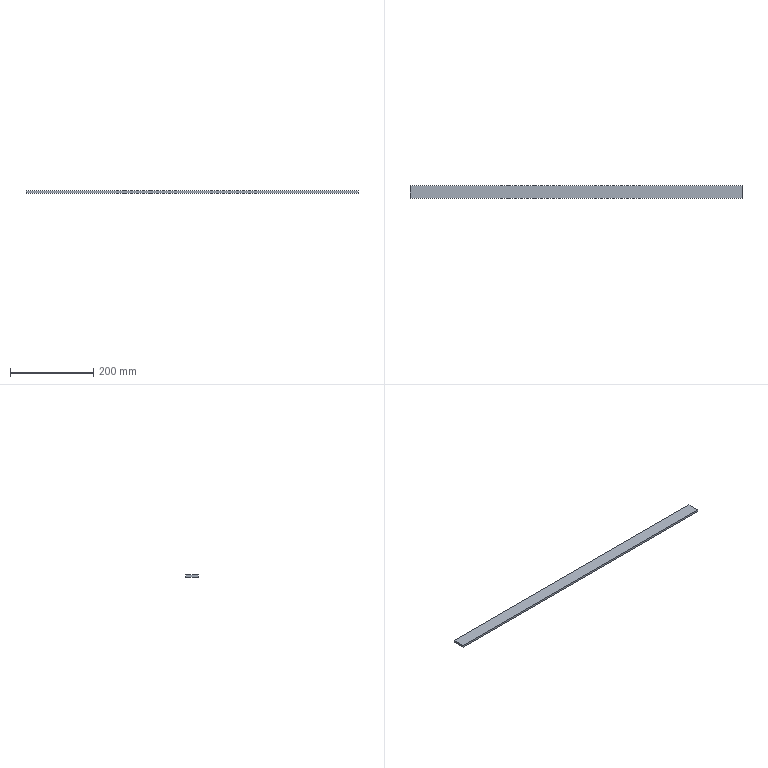Part | SolidWorks | features Extrusion 1 | 1 solid | 6 faces | box 800 x 30 x 5 mm | volume 120000 mm3 | plane 6
STEP:
#1=CARTESIAN_POINT('',(400.,-15.,0.));
#2=VERTEX_POINT('',#1);
#3=CARTESIAN_POINT('',(400.,15.,0.));
#4=VERTEX_POINT('',#3);
#5=CARTESIAN_POINT('',(400.,15.,0.));
#6=DIRECTION('',(0.,1.,0.));
#7=VECTOR('',#6,1000.);
#8=LINE('',#5,#7);
#9=EDGE_CURVE('',#2,#4,#8,.T.);
#10=ORIENTED_EDGE('',*,*,#9,.T.);
#11=CARTESIAN_POINT('',(400.,15.,5.));
#12=VERTEX_POINT('',#11);
#13=CARTESIAN_POINT('',(400.,15.,5.));
#14=DIRECTION('',(0.,0.,-1.));
#15=VECTOR('',#14,1000.);
#16=LINE('',#13,#15);
#17=EDGE_CURVE('',#12,#4,#16,.T.);
#18=ORIENTED_EDGE('',*,*,#17,.F.);
#19=CARTESIAN_POINT('',(400.,-15.,5.));
#20=VERTEX_POINT('',#19);
#21=CARTESIAN_POINT('',(400.,15.,5.));
#22=DIRECTION('',(0.,1.,0.));
#23=VECTOR('',#22,1000.);
#24=LINE('',#21,#23);
#25=EDGE_CURVE('',#20,#12,#24,.T.);
#26=ORIENTED_EDGE('',*,*,#25,.F.);
#27=CARTESIAN_POINT('',(400.,-15.,5.));
#28=DIRECTION('',(0.,0.,-1.));
#29=VECTOR('',#28,1000.);
#30=LINE('',#27,#29);
#31=EDGE_CURVE('',#20,#2,#30,.T.);
#32=ORIENTED_EDGE('',*,*,#31,.T.);
#33=EDGE_LOOP('',(#10,#18,#26,#32));
#34=FACE_OUTER_BOUND('',#33,.T.);
#35=CARTESIAN_POINT('',(400.,15.,5.));
#36=DIRECTION('',(-1.,0.,0.));
#37=DIRECTION('',(0.,0.,1.));
#38=AXIS2_PLACEMENT_3D('',#35,#36,#37);
#39=PLANE('',#38);
#40=ADVANCED_FACE('',(#34),#39,.F.);
#41=CARTESIAN_POINT('',(-400.,15.,0.));
#42=VERTEX_POINT('',#41);
#43=CARTESIAN_POINT('',(-400.,15.,0.));
#44=DIRECTION('',(-1.,0.,0.));
#45=VECTOR('',#44,1000.);
#46=LINE('',#43,#45);
#47=EDGE_CURVE('',#4,#42,#46,.T.);
#48=ORIENTED_EDGE('',*,*,#47,.T.);
#49=CARTESIAN_POINT('',(-400.,15.,5.));
#50=VERTEX_POINT('',#49);
#51=CARTESIAN_POINT('',(-400.,15.,5.));
#52=DIRECTION('',(0.,0.,-1.));
#53=VECTOR('',#52,1000.);
#54=LINE('',#51,#53);
#55=EDGE_CURVE('',#50,#42,#54,.T.);
#56=ORIENTED_EDGE('',*,*,#55,.F.);
#57=CARTESIAN_POINT('',(-400.,15.,5.));
#58=DIRECTION('',(-1.,0.,0.));
#59=VECTOR('',#58,1000.);
#60=LINE('',#57,#59);
#61=EDGE_CURVE('',#12,#50,#60,.T.);
#62=ORIENTED_EDGE('',*,*,#61,.F.);
#63=ORIENTED_EDGE('',*,*,#17,.T.);
#64=EDGE_LOOP('',(#48,#56,#62,#63));
#65=FACE_OUTER_BOUND('',#64,.T.);
#66=CARTESIAN_POINT('',(-400.,15.,5.));
#67=DIRECTION('',(0.,-1.,0.));
#68=DIRECTION('',(0.,0.,-1.));
#69=AXIS2_PLACEMENT_3D('',#66,#67,#68);
#70=PLANE('',#69);
#71=ADVANCED_FACE('',(#65),#70,.F.);
#72=CARTESIAN_POINT('',(-400.,-15.,0.));
#73=VERTEX_POINT('',#72);
#74=CARTESIAN_POINT('',(-400.,15.,0.));
#75=DIRECTION('',(0.,-1.,0.));
#76=VECTOR('',#75,1000.);
#77=LINE('',#74,#76);
#78=EDGE_CURVE('',#42,#73,#77,.T.);
#79=ORIENTED_EDGE('',*,*,#78,.T.);
#80=CARTESIAN_POINT('',(-400.,-15.,5.));
#81=VERTEX_POINT('',#80);
#82=CARTESIAN_POINT('',(-400.,-15.,5.));
#83=DIRECTION('',(0.,0.,-1.));
#84=VECTOR('',#83,1000.);
#85=LINE('',#82,#84);
#86=EDGE_CURVE('',#81,#73,#85,.T.);
#87=ORIENTED_EDGE('',*,*,#86,.F.);
#88=CARTESIAN_POINT('',(-400.,15.,5.));
#89=DIRECTION('',(0.,-1.,0.));
#90=VECTOR('',#89,1000.);
#91=LINE('',#88,#90);
#92=EDGE_CURVE('',#50,#81,#91,.T.);
#93=ORIENTED_EDGE('',*,*,#92,.F.);
#94=ORIENTED_EDGE('',*,*,#55,.T.);
#95=EDGE_LOOP('',(#79,#87,#93,#94));
#96=FACE_OUTER_BOUND('',#95,.T.);
#97=CARTESIAN_POINT('',(-400.,15.,5.));
#98=DIRECTION('',(1.,0.,0.));
#99=DIRECTION('',(0.,0.,-1.));
#100=AXIS2_PLACEMENT_3D('',#97,#98,#99);
#101=PLANE('',#100);
#102=ADVANCED_FACE('',(#96),#101,.F.);
#103=CARTESIAN_POINT('',(-400.,-15.,0.));
#104=DIRECTION('',(1.,0.,0.));
#105=VECTOR('',#104,1000.);
#106=LINE('',#103,#105);
#107=EDGE_CURVE('',#73,#2,#106,.T.);
#108=ORIENTED_EDGE('',*,*,#107,.T.);
#109=ORIENTED_EDGE('',*,*,#31,.F.);
#110=CARTESIAN_POINT('',(-400.,-15.,5.));
#111=DIRECTION('',(1.,0.,0.));
#112=VECTOR('',#111,1000.);
#113=LINE('',#110,#112);
#114=EDGE_CURVE('',#81,#20,#113,.T.);
#115=ORIENTED_EDGE('',*,*,#114,.F.);
#116=ORIENTED_EDGE('',*,*,#86,.T.);
#117=EDGE_LOOP('',(#108,#109,#115,#116));
#118=FACE_OUTER_BOUND('',#117,.T.);
#119=CARTESIAN_POINT('',(-400.,-15.,5.));
#120=DIRECTION('',(0.,1.,0.));
#121=DIRECTION('',(0.,0.,1.));
#122=AXIS2_PLACEMENT_3D('',#119,#120,#121);
#123=PLANE('',#122);
#124=ADVANCED_FACE('',(#118),#123,.F.);
#125=ORIENTED_EDGE('',*,*,#25,.T.);
#126=ORIENTED_EDGE('',*,*,#61,.T.);
#127=ORIENTED_EDGE('',*,*,#92,.T.);
#128=ORIENTED_EDGE('',*,*,#114,.T.);
#129=EDGE_LOOP('',(#125,#126,#127,#128));
#130=FACE_OUTER_BOUND('',#129,.T.);
#131=CARTESIAN_POINT('',(0.,0.,5.));
#132=DIRECTION('',(0.,0.,1.));
#133=DIRECTION('',(1.,0.,0.));
#134=AXIS2_PLACEMENT_3D('',#131,#132,#133);
#135=PLANE('',#134);
#136=ADVANCED_FACE('',(#130),#135,.T.);
#137=ORIENTED_EDGE('',*,*,#9,.F.);
#138=ORIENTED_EDGE('',*,*,#107,.F.);
#139=ORIENTED_EDGE('',*,*,#78,.F.);
#140=ORIENTED_EDGE('',*,*,#47,.F.);
#141=EDGE_LOOP('',(#137,#138,#139,#140));
#142=FACE_OUTER_BOUND('',#141,.T.);
#143=CARTESIAN_POINT('',(0.,0.,0.));
#144=DIRECTION('',(0.,0.,1.));
#145=DIRECTION('',(1.,0.,0.));
#146=AXIS2_PLACEMENT_3D('',#143,#144,#145);
#147=PLANE('',#146);
#148=ADVANCED_FACE('',(#142),#147,.F.);
#149=CLOSED_SHELL('',(#40,#71,#102,#124,#136,#148));
#150=MANIFOLD_SOLID_BREP('',#149);
#151=CARTESIAN_POINT('',(0.,0.,0.));
#152=DIRECTION('',(0.,0.,1.));
#153=DIRECTION('',(1.,0.,0.));
#154=AXIS2_PLACEMENT_3D('',#151,#152,#153);
#155=(LENGTH_UNIT()NAMED_UNIT(*)SI_UNIT(.MILLI.,.METRE.));
#156=UNCERTAINTY_MEASURE_WITH_UNIT(LENGTH_MEASURE(0.00001),#155,'','');
#157=(NAMED_UNIT(*)PLANE_ANGLE_UNIT()SI_UNIT($,.RADIAN.));
#158=(NAMED_UNIT(*)SI_UNIT($,.STERADIAN.)SOLID_ANGLE_UNIT());
#159=(GEOMETRIC_REPRESENTATION_CONTEXT(3)GLOBAL_UNCERTAINTY_ASSIGNED_CONTEXT((#156))GLOBAL_UNIT_ASSIGNED_CONTEXT((#155,#157,#158))REPRESENTATION_CONTEXT('',''));
#160=ADVANCED_BREP_SHAPE_REPRESENTATION('',(#150,#154),#159);